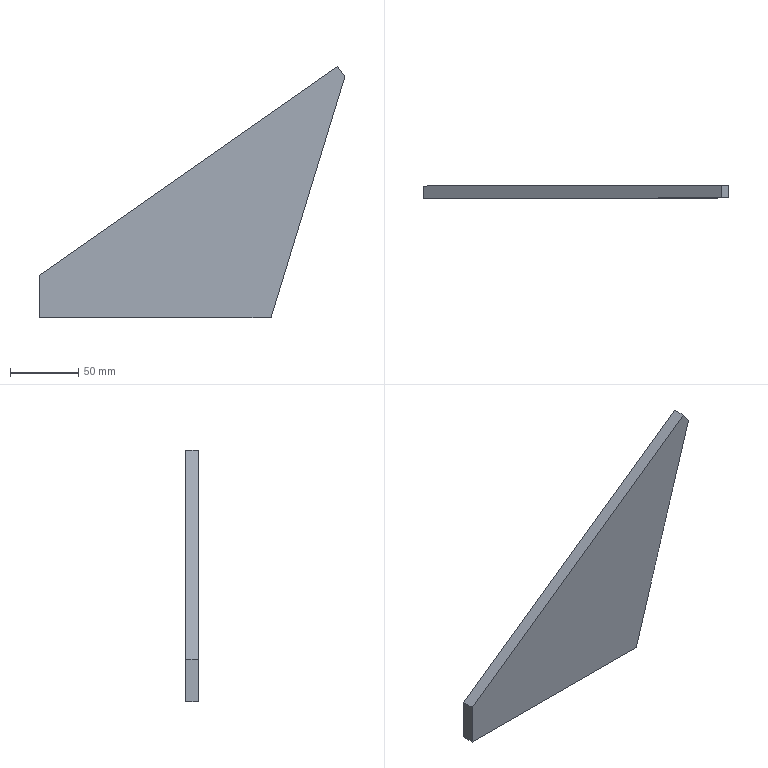Part | SolidWorks | features FlatPattern 1, SMBaseFlange 1, SheetMetal 1 | 1 solid | 7 faces | box 224.107 x 9 x 184.117 mm | volume 177492 mm3 | plane 7
STEP:
#1=CARTESIAN_POINT('',(0.,0.,0.));
#2=VERTEX_POINT('',#1);
#3=CARTESIAN_POINT('',(0.,0.,31.));
#4=VERTEX_POINT('',#3);
#5=CARTESIAN_POINT('',(0.,0.,31.));
#6=DIRECTION('',(0.,0.,1.));
#7=VECTOR('',#6,1000.);
#8=LINE('',#5,#7);
#9=EDGE_CURVE('',#2,#4,#8,.T.);
#10=ORIENTED_EDGE('',*,*,#9,.F.);
#11=CARTESIAN_POINT('',(0.,-9.,0.));
#12=VERTEX_POINT('',#11);
#13=CARTESIAN_POINT('',(0.,-9.,0.));
#14=DIRECTION('',(0.,1.,0.));
#15=VECTOR('',#14,1000.);
#16=LINE('',#13,#15);
#17=EDGE_CURVE('',#12,#2,#16,.T.);
#18=ORIENTED_EDGE('',*,*,#17,.F.);
#19=CARTESIAN_POINT('',(0.,-9.,31.));
#20=VERTEX_POINT('',#19);
#21=CARTESIAN_POINT('',(0.,-9.,31.));
#22=DIRECTION('',(0.,0.,1.));
#23=VECTOR('',#22,1000.);
#24=LINE('',#21,#23);
#25=EDGE_CURVE('',#12,#20,#24,.T.);
#26=ORIENTED_EDGE('',*,*,#25,.T.);
#27=CARTESIAN_POINT('',(0.,-9.,31.));
#28=DIRECTION('',(0.,1.,0.));
#29=VECTOR('',#28,1000.);
#30=LINE('',#27,#29);
#31=EDGE_CURVE('',#20,#4,#30,.T.);
#32=ORIENTED_EDGE('',*,*,#31,.T.);
#33=EDGE_LOOP('',(#10,#18,#26,#32));
#34=FACE_OUTER_BOUND('',#33,.T.);
#35=CARTESIAN_POINT('',(0.,-9.,31.));
#36=DIRECTION('',(-1.,0.,0.));
#37=DIRECTION('',(0.,0.,1.));
#38=AXIS2_PLACEMENT_3D('',#35,#36,#37);
#39=PLANE('',#38);
#40=ADVANCED_FACE('',(#34),#39,.T.);
#41=CARTESIAN_POINT('',(170.,0.,0.));
#42=VERTEX_POINT('',#41);
#43=CARTESIAN_POINT('',(0.,0.,0.));
#44=DIRECTION('',(-1.,0.,0.));
#45=VECTOR('',#44,1000.);
#46=LINE('',#43,#45);
#47=EDGE_CURVE('',#42,#2,#46,.T.);
#48=ORIENTED_EDGE('',*,*,#47,.F.);
#49=CARTESIAN_POINT('',(170.,-9.,0.));
#50=VERTEX_POINT('',#49);
#51=CARTESIAN_POINT('',(170.,-9.,0.));
#52=DIRECTION('',(0.,1.,0.));
#53=VECTOR('',#52,1000.);
#54=LINE('',#51,#53);
#55=EDGE_CURVE('',#50,#42,#54,.T.);
#56=ORIENTED_EDGE('',*,*,#55,.F.);
#57=CARTESIAN_POINT('',(0.,-9.,0.));
#58=DIRECTION('',(-1.,0.,0.));
#59=VECTOR('',#58,1000.);
#60=LINE('',#57,#59);
#61=EDGE_CURVE('',#50,#12,#60,.T.);
#62=ORIENTED_EDGE('',*,*,#61,.T.);
#63=ORIENTED_EDGE('',*,*,#17,.T.);
#64=EDGE_LOOP('',(#48,#56,#62,#63));
#65=FACE_OUTER_BOUND('',#64,.T.);
#66=CARTESIAN_POINT('',(0.,-9.,0.));
#67=DIRECTION('',(0.,0.,-1.));
#68=DIRECTION('',(-1.,0.,0.));
#69=AXIS2_PLACEMENT_3D('',#66,#67,#68);
#70=PLANE('',#69);
#71=ADVANCED_FACE('',(#65),#70,.T.);
#72=CARTESIAN_POINT('',(224.107,0.,176.658));
#73=VERTEX_POINT('',#72);
#74=CARTESIAN_POINT('',(170.,0.,0.));
#75=DIRECTION('',(-0.2929,0.,-0.9562));
#76=VECTOR('',#75,1000.);
#77=LINE('',#74,#76);
#78=EDGE_CURVE('',#73,#42,#77,.T.);
#79=ORIENTED_EDGE('',*,*,#78,.F.);
#80=CARTESIAN_POINT('',(224.107,-9.,176.658));
#81=VERTEX_POINT('',#80);
#82=CARTESIAN_POINT('',(224.107,-9.,176.658));
#83=DIRECTION('',(0.,1.,0.));
#84=VECTOR('',#83,1000.);
#85=LINE('',#82,#84);
#86=EDGE_CURVE('',#81,#73,#85,.T.);
#87=ORIENTED_EDGE('',*,*,#86,.F.);
#88=CARTESIAN_POINT('',(170.,-9.,0.));
#89=DIRECTION('',(-0.2929,0.,-0.9562));
#90=VECTOR('',#89,1000.);
#91=LINE('',#88,#90);
#92=EDGE_CURVE('',#81,#50,#91,.T.);
#93=ORIENTED_EDGE('',*,*,#92,.T.);
#94=ORIENTED_EDGE('',*,*,#55,.T.);
#95=EDGE_LOOP('',(#79,#87,#93,#94));
#96=FACE_OUTER_BOUND('',#95,.T.);
#97=CARTESIAN_POINT('',(170.,-9.,0.));
#98=DIRECTION('',(0.9562,0.,-0.2929));
#99=DIRECTION('',(-0.2929,0.,-0.9562));
#100=AXIS2_PLACEMENT_3D('',#97,#98,#99);
#101=PLANE('',#100);
#102=ADVANCED_FACE('',(#96),#101,.T.);
#103=CARTESIAN_POINT('',(218.67,0.,184.117));
#104=VERTEX_POINT('',#103);
#105=CARTESIAN_POINT('',(218.67,0.,184.117));
#106=DIRECTION('',(0.589,0.,-0.8081));
#107=VECTOR('',#106,1000.);
#108=LINE('',#105,#107);
#109=EDGE_CURVE('',#104,#73,#108,.T.);
#110=ORIENTED_EDGE('',*,*,#109,.F.);
#111=CARTESIAN_POINT('',(218.67,-9.,184.117));
#112=VERTEX_POINT('',#111);
#113=CARTESIAN_POINT('',(218.67,-9.,184.117));
#114=DIRECTION('',(0.,1.,0.));
#115=VECTOR('',#114,1000.);
#116=LINE('',#113,#115);
#117=EDGE_CURVE('',#112,#104,#116,.T.);
#118=ORIENTED_EDGE('',*,*,#117,.F.);
#119=CARTESIAN_POINT('',(218.67,-9.,184.117));
#120=DIRECTION('',(0.589,0.,-0.8081));
#121=VECTOR('',#120,1000.);
#122=LINE('',#119,#121);
#123=EDGE_CURVE('',#112,#81,#122,.T.);
#124=ORIENTED_EDGE('',*,*,#123,.T.);
#125=ORIENTED_EDGE('',*,*,#86,.T.);
#126=EDGE_LOOP('',(#110,#118,#124,#125));
#127=FACE_OUTER_BOUND('',#126,.T.);
#128=CARTESIAN_POINT('',(218.67,-9.,184.117));
#129=DIRECTION('',(0.8081,0.,0.589));
#130=DIRECTION('',(0.589,0.,-0.8081));
#131=AXIS2_PLACEMENT_3D('',#128,#129,#130);
#132=PLANE('',#131);
#133=ADVANCED_FACE('',(#127),#132,.T.);
#134=CARTESIAN_POINT('',(218.67,0.,184.117));
#135=DIRECTION('',(0.8191,0.,0.5736));
#136=VECTOR('',#135,1000.);
#137=LINE('',#134,#136);
#138=EDGE_CURVE('',#4,#104,#137,.T.);
#139=ORIENTED_EDGE('',*,*,#138,.F.);
#140=ORIENTED_EDGE('',*,*,#31,.F.);
#141=CARTESIAN_POINT('',(218.67,-9.,184.117));
#142=DIRECTION('',(0.8191,0.,0.5736));
#143=VECTOR('',#142,1000.);
#144=LINE('',#141,#143);
#145=EDGE_CURVE('',#20,#112,#144,.T.);
#146=ORIENTED_EDGE('',*,*,#145,.T.);
#147=ORIENTED_EDGE('',*,*,#117,.T.);
#148=EDGE_LOOP('',(#139,#140,#146,#147));
#149=FACE_OUTER_BOUND('',#148,.T.);
#150=CARTESIAN_POINT('',(218.67,-9.,184.117));
#151=DIRECTION('',(-0.5736,0.,0.8191));
#152=DIRECTION('',(0.8191,0.,0.5736));
#153=AXIS2_PLACEMENT_3D('',#150,#151,#152);
#154=PLANE('',#153);
#155=ADVANCED_FACE('',(#149),#154,.T.);
#156=ORIENTED_EDGE('',*,*,#25,.F.);
#157=ORIENTED_EDGE('',*,*,#61,.F.);
#158=ORIENTED_EDGE('',*,*,#92,.F.);
#159=ORIENTED_EDGE('',*,*,#123,.F.);
#160=ORIENTED_EDGE('',*,*,#145,.F.);
#161=EDGE_LOOP('',(#156,#157,#158,#159,#160));
#162=FACE_OUTER_BOUND('',#161,.T.);
#163=CARTESIAN_POINT('',(0.,-9.,0.));
#164=DIRECTION('',(0.,-1.,0.));
#165=DIRECTION('',(0.,0.,-1.));
#166=AXIS2_PLACEMENT_3D('',#163,#164,#165);
#167=PLANE('',#166);
#168=ADVANCED_FACE('',(#162),#167,.T.);
#169=ORIENTED_EDGE('',*,*,#9,.T.);
#170=ORIENTED_EDGE('',*,*,#138,.T.);
#171=ORIENTED_EDGE('',*,*,#109,.T.);
#172=ORIENTED_EDGE('',*,*,#78,.T.);
#173=ORIENTED_EDGE('',*,*,#47,.T.);
#174=EDGE_LOOP('',(#169,#170,#171,#172,#173));
#175=FACE_OUTER_BOUND('',#174,.T.);
#176=CARTESIAN_POINT('',(0.,0.,0.));
#177=DIRECTION('',(0.,-1.,0.));
#178=DIRECTION('',(0.,0.,-1.));
#179=AXIS2_PLACEMENT_3D('',#176,#177,#178);
#180=PLANE('',#179);
#181=ADVANCED_FACE('',(#175),#180,.F.);
#182=CLOSED_SHELL('',(#40,#71,#102,#133,#155,#168,#181));
#183=MANIFOLD_SOLID_BREP('',#182);
#184=CARTESIAN_POINT('',(0.,0.,0.));
#185=DIRECTION('',(0.,0.,1.));
#186=DIRECTION('',(1.,0.,0.));
#187=AXIS2_PLACEMENT_3D('',#184,#185,#186);
#188=(LENGTH_UNIT()NAMED_UNIT(*)SI_UNIT(.MILLI.,.METRE.));
#189=UNCERTAINTY_MEASURE_WITH_UNIT(LENGTH_MEASURE(0.00001),#188,'','');
#190=(NAMED_UNIT(*)PLANE_ANGLE_UNIT()SI_UNIT($,.RADIAN.));
#191=(NAMED_UNIT(*)SI_UNIT($,.STERADIAN.)SOLID_ANGLE_UNIT());
#192=(GEOMETRIC_REPRESENTATION_CONTEXT(3)GLOBAL_UNCERTAINTY_ASSIGNED_CONTEXT((#189))GLOBAL_UNIT_ASSIGNED_CONTEXT((#188,#190,#191))REPRESENTATION_CONTEXT('',''));
#193=ADVANCED_BREP_SHAPE_REPRESENTATION('',(#183,#187),#192);